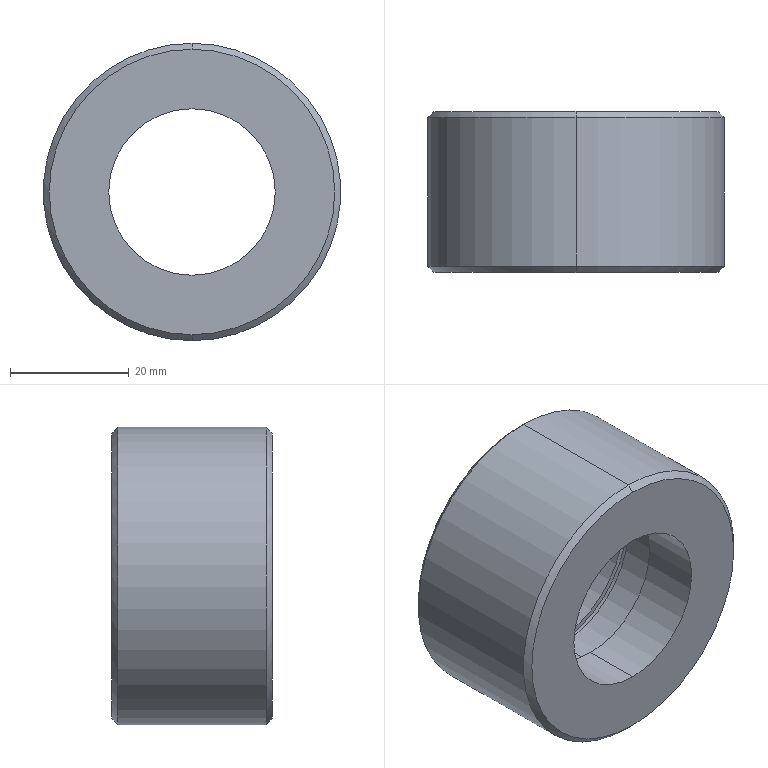Part | SolidWorks | features Chamfer 2, ICE 2, Extrusion 1, RevCut 1 | 1 solid | 21 faces | box 50 x 27 x 50 mm | volume 32903 mm3 | cylinder 10 | cone 6 | plane 5 | commonest cylinder face diameters 32 x4 28 x2 33.7 x2 50 x2
STEP:
#1=CARTESIAN_POINT('',(0.,17.,-16.85));
#2=VERTEX_POINT('',#1);
#3=CARTESIAN_POINT('',(0.,17.,16.85));
#4=VERTEX_POINT('',#3);
#5=CARTESIAN_POINT('',(0.,17.,0.));
#6=DIRECTION('',(0.,1.,0.));
#7=DIRECTION('',(0.,0.,1.));
#8=AXIS2_PLACEMENT_3D('',#5,#6,#7);
#9=CIRCLE('',#8,16.85);
#10=EDGE_CURVE('',#2,#4,#9,.T.);
#11=ORIENTED_EDGE('',*,*,#10,.F.);
#12=CARTESIAN_POINT('',(0.,18.3,-16.85));
#13=VERTEX_POINT('',#12);
#14=CARTESIAN_POINT('',(0.,26.,-16.85));
#15=DIRECTION('',(0.,1.,0.));
#16=VECTOR('',#15,1000.);
#17=LINE('',#14,#16);
#18=EDGE_CURVE('',#2,#13,#17,.T.);
#19=ORIENTED_EDGE('',*,*,#18,.T.);
#20=CARTESIAN_POINT('',(0.,18.3,16.85));
#21=VERTEX_POINT('',#20);
#22=CARTESIAN_POINT('',(0.,18.3,0.));
#23=DIRECTION('',(0.,1.,0.));
#24=DIRECTION('',(0.,0.,1.));
#25=AXIS2_PLACEMENT_3D('',#22,#23,#24);
#26=CIRCLE('',#25,16.85);
#27=EDGE_CURVE('',#13,#21,#26,.T.);
#28=ORIENTED_EDGE('',*,*,#27,.T.);
#29=CARTESIAN_POINT('',(0.,26.,16.85));
#30=DIRECTION('',(0.,1.,0.));
#31=VECTOR('',#30,1000.);
#32=LINE('',#29,#31);
#33=EDGE_CURVE('',#4,#21,#32,.T.);
#34=ORIENTED_EDGE('',*,*,#33,.F.);
#35=EDGE_LOOP('',(#11,#19,#28,#34));
#36=FACE_OUTER_BOUND('',#35,.T.);
#37=CARTESIAN_POINT('',(0.,26.,0.));
#38=DIRECTION('',(0.,1.,0.));
#39=DIRECTION('',(0.,0.,1.));
#40=AXIS2_PLACEMENT_3D('',#37,#38,#39);
#41=CYLINDRICAL_SURFACE('',#40,16.85);
#42=ADVANCED_FACE('',(#36),#41,.F.);
#43=CARTESIAN_POINT('',(0.,26.5,-16.));
#44=VERTEX_POINT('',#43);
#45=CARTESIAN_POINT('',(0.,26.5,16.));
#46=VERTEX_POINT('',#45);
#47=CARTESIAN_POINT('',(0.,26.5,0.));
#48=DIRECTION('',(0.,1.,0.));
#49=DIRECTION('',(0.,0.,1.));
#50=AXIS2_PLACEMENT_3D('',#47,#48,#49);
#51=CIRCLE('',#50,16.);
#52=EDGE_CURVE('',#44,#46,#51,.T.);
#53=ORIENTED_EDGE('',*,*,#52,.F.);
#54=CARTESIAN_POINT('',(0.,27.,-16.5));
#55=VERTEX_POINT('',#54);
#56=CARTESIAN_POINT('',(0.,26.5,-16.));
#57=DIRECTION('',(0.,0.7071,-0.7071));
#58=VECTOR('',#57,1000.);
#59=LINE('',#56,#58);
#60=EDGE_CURVE('',#44,#55,#59,.T.);
#61=ORIENTED_EDGE('',*,*,#60,.T.);
#62=CARTESIAN_POINT('',(0.,27.,16.5));
#63=VERTEX_POINT('',#62);
#64=CARTESIAN_POINT('',(0.,27.,0.));
#65=DIRECTION('',(0.,-1.,0.));
#66=DIRECTION('',(0.,0.,1.));
#67=AXIS2_PLACEMENT_3D('',#64,#65,#66);
#68=CIRCLE('',#67,16.5);
#69=EDGE_CURVE('',#63,#55,#68,.T.);
#70=ORIENTED_EDGE('',*,*,#69,.F.);
#71=CARTESIAN_POINT('',(0.,26.5,16.));
#72=DIRECTION('',(0.,0.7071,0.7071));
#73=VECTOR('',#72,1000.);
#74=LINE('',#71,#73);
#75=EDGE_CURVE('',#46,#63,#74,.T.);
#76=ORIENTED_EDGE('',*,*,#75,.F.);
#77=EDGE_LOOP('',(#53,#61,#70,#76));
#78=FACE_OUTER_BOUND('',#77,.T.);
#79=CARTESIAN_POINT('',(0.,26.5,0.));
#80=DIRECTION('',(0.,1.,0.));
#81=DIRECTION('',(0.,0.,1.));
#82=AXIS2_PLACEMENT_3D('',#79,#80,#81);
#83=CONICAL_SURFACE('',#82,16.,0.7854);
#84=ADVANCED_FACE('',(#78),#83,.F.);
#85=CARTESIAN_POINT('',(0.,27.,24.));
#86=VERTEX_POINT('',#85);
#87=CARTESIAN_POINT('',(0.,27.,-24.));
#88=VERTEX_POINT('',#87);
#89=CARTESIAN_POINT('',(0.,27.,0.));
#90=DIRECTION('',(0.,1.,0.));
#91=DIRECTION('',(0.,0.,1.));
#92=AXIS2_PLACEMENT_3D('',#89,#90,#91);
#93=CIRCLE('',#92,24.);
#94=EDGE_CURVE('',#86,#88,#93,.T.);
#95=ORIENTED_EDGE('',*,*,#94,.F.);
#96=CARTESIAN_POINT('',(0.,26.,25.));
#97=VERTEX_POINT('',#96);
#98=CARTESIAN_POINT('',(0.,27.,24.));
#99=DIRECTION('',(0.,-0.7071,0.7071));
#100=VECTOR('',#99,1000.);
#101=LINE('',#98,#100);
#102=EDGE_CURVE('',#86,#97,#101,.T.);
#103=ORIENTED_EDGE('',*,*,#102,.T.);
#104=CARTESIAN_POINT('',(0.,26.,-25.));
#105=VERTEX_POINT('',#104);
#106=CARTESIAN_POINT('',(0.,26.,0.));
#107=DIRECTION('',(0.,-1.,0.));
#108=DIRECTION('',(0.,0.,1.));
#109=AXIS2_PLACEMENT_3D('',#106,#107,#108);
#110=CIRCLE('',#109,25.);
#111=EDGE_CURVE('',#105,#97,#110,.T.);
#112=ORIENTED_EDGE('',*,*,#111,.F.);
#113=CARTESIAN_POINT('',(0.,27.,-24.));
#114=DIRECTION('',(0.,-0.7071,-0.7071));
#115=VECTOR('',#114,1000.);
#116=LINE('',#113,#115);
#117=EDGE_CURVE('',#88,#105,#116,.T.);
#118=ORIENTED_EDGE('',*,*,#117,.F.);
#119=EDGE_LOOP('',(#95,#103,#112,#118));
#120=FACE_OUTER_BOUND('',#119,.T.);
#121=CARTESIAN_POINT('',(0.,27.,0.));
#122=DIRECTION('',(0.,-1.,0.));
#123=DIRECTION('',(0.,0.,-1.));
#124=AXIS2_PLACEMENT_3D('',#121,#122,#123);
#125=CONICAL_SURFACE('',#124,24.,0.7854);
#126=ADVANCED_FACE('',(#120),#125,.T.);
#127=CARTESIAN_POINT('',(0.,0.,-24.));
#128=VERTEX_POINT('',#127);
#129=CARTESIAN_POINT('',(0.,0.,24.));
#130=VERTEX_POINT('',#129);
#131=CARTESIAN_POINT('',(0.,0.,0.));
#132=DIRECTION('',(0.,-1.,0.));
#133=DIRECTION('',(0.,0.,1.));
#134=AXIS2_PLACEMENT_3D('',#131,#132,#133);
#135=CIRCLE('',#134,24.);
#136=EDGE_CURVE('',#128,#130,#135,.T.);
#137=ORIENTED_EDGE('',*,*,#136,.F.);
#138=CARTESIAN_POINT('',(0.,1.,-25.));
#139=VERTEX_POINT('',#138);
#140=CARTESIAN_POINT('',(0.,1.,-25.));
#141=DIRECTION('',(0.,0.7071,-0.7071));
#142=VECTOR('',#141,1000.);
#143=LINE('',#140,#142);
#144=EDGE_CURVE('',#128,#139,#143,.T.);
#145=ORIENTED_EDGE('',*,*,#144,.T.);
#146=CARTESIAN_POINT('',(0.,1.,25.));
#147=VERTEX_POINT('',#146);
#148=CARTESIAN_POINT('',(0.,1.,0.));
#149=DIRECTION('',(0.,1.,0.));
#150=DIRECTION('',(0.,0.,1.));
#151=AXIS2_PLACEMENT_3D('',#148,#149,#150);
#152=CIRCLE('',#151,25.);
#153=EDGE_CURVE('',#147,#139,#152,.T.);
#154=ORIENTED_EDGE('',*,*,#153,.F.);
#155=CARTESIAN_POINT('',(0.,1.,25.));
#156=DIRECTION('',(0.,0.7071,0.7071));
#157=VECTOR('',#156,1000.);
#158=LINE('',#155,#157);
#159=EDGE_CURVE('',#130,#147,#158,.T.);
#160=ORIENTED_EDGE('',*,*,#159,.F.);
#161=EDGE_LOOP('',(#137,#145,#154,#160));
#162=FACE_OUTER_BOUND('',#161,.T.);
#163=CARTESIAN_POINT('',(0.,1.,0.));
#164=DIRECTION('',(0.,1.,0.));
#165=DIRECTION('',(0.,0.,1.));
#166=AXIS2_PLACEMENT_3D('',#163,#164,#165);
#167=CONICAL_SURFACE('',#166,25.,0.7854);
#168=ADVANCED_FACE('',(#162),#167,.T.);
#169=CARTESIAN_POINT('',(0.,0.,-14.));
#170=VERTEX_POINT('',#169);
#171=CARTESIAN_POINT('',(0.,0.,14.));
#172=VERTEX_POINT('',#171);
#173=CARTESIAN_POINT('',(0.,0.,0.));
#174=DIRECTION('',(0.,1.,0.));
#175=DIRECTION('',(0.,0.,1.));
#176=AXIS2_PLACEMENT_3D('',#173,#174,#175);
#177=CIRCLE('',#176,14.);
#178=EDGE_CURVE('',#170,#172,#177,.T.);
#179=ORIENTED_EDGE('',*,*,#178,.F.);
#180=CARTESIAN_POINT('',(0.,10.,-14.));
#181=VERTEX_POINT('',#180);
#182=CARTESIAN_POINT('',(0.,0.,-14.));
#183=DIRECTION('',(0.,1.,0.));
#184=VECTOR('',#183,1000.);
#185=LINE('',#182,#184);
#186=EDGE_CURVE('',#170,#181,#185,.T.);
#187=ORIENTED_EDGE('',*,*,#186,.T.);
#188=CARTESIAN_POINT('',(0.,10.,14.));
#189=VERTEX_POINT('',#188);
#190=CARTESIAN_POINT('',(0.,10.,0.));
#191=DIRECTION('',(0.,1.,0.));
#192=DIRECTION('',(0.,0.,1.));
#193=AXIS2_PLACEMENT_3D('',#190,#191,#192);
#194=CIRCLE('',#193,14.);
#195=EDGE_CURVE('',#181,#189,#194,.T.);
#196=ORIENTED_EDGE('',*,*,#195,.T.);
#197=CARTESIAN_POINT('',(0.,0.,14.));
#198=DIRECTION('',(0.,1.,0.));
#199=VECTOR('',#198,1000.);
#200=LINE('',#197,#199);
#201=EDGE_CURVE('',#172,#189,#200,.T.);
#202=ORIENTED_EDGE('',*,*,#201,.F.);
#203=EDGE_LOOP('',(#179,#187,#196,#202));
#204=FACE_OUTER_BOUND('',#203,.T.);
#205=CARTESIAN_POINT('',(0.,0.,0.));
#206=DIRECTION('',(0.,1.,0.));
#207=DIRECTION('',(0.,0.,1.));
#208=AXIS2_PLACEMENT_3D('',#205,#206,#207);
#209=CYLINDRICAL_SURFACE('',#208,14.);
#210=ADVANCED_FACE('',(#204),#209,.F.);
#211=CARTESIAN_POINT('',(0.,10.,-16.));
#212=VERTEX_POINT('',#211);
#213=CARTESIAN_POINT('',(0.,10.,16.));
#214=VERTEX_POINT('',#213);
#215=CARTESIAN_POINT('',(0.,10.,0.));
#216=DIRECTION('',(0.,1.,0.));
#217=DIRECTION('',(0.,0.,1.));
#218=AXIS2_PLACEMENT_3D('',#215,#216,#217);
#219=CIRCLE('',#218,16.);
#220=EDGE_CURVE('',#212,#214,#219,.T.);
#221=ORIENTED_EDGE('',*,*,#220,.F.);
#222=CARTESIAN_POINT('',(0.,17.,-16.));
#223=VERTEX_POINT('',#222);
#224=CARTESIAN_POINT('',(0.,10.,-16.));
#225=DIRECTION('',(0.,1.,0.));
#226=VECTOR('',#225,1000.);
#227=LINE('',#224,#226);
#228=EDGE_CURVE('',#212,#223,#227,.T.);
#229=ORIENTED_EDGE('',*,*,#228,.T.);
#230=CARTESIAN_POINT('',(0.,17.,16.));
#231=VERTEX_POINT('',#230);
#232=CARTESIAN_POINT('',(0.,17.,0.));
#233=DIRECTION('',(0.,1.,0.));
#234=DIRECTION('',(0.,0.,-1.));
#235=AXIS2_PLACEMENT_3D('',#232,#233,#234);
#236=CIRCLE('',#235,16.);
#237=EDGE_CURVE('',#223,#231,#236,.T.);
#238=ORIENTED_EDGE('',*,*,#237,.T.);
#239=CARTESIAN_POINT('',(0.,10.,16.));
#240=DIRECTION('',(0.,1.,0.));
#241=VECTOR('',#240,1000.);
#242=LINE('',#239,#241);
#243=EDGE_CURVE('',#214,#231,#242,.T.);
#244=ORIENTED_EDGE('',*,*,#243,.F.);
#245=EDGE_LOOP('',(#221,#229,#238,#244));
#246=FACE_OUTER_BOUND('',#245,.T.);
#247=CARTESIAN_POINT('',(0.,10.,0.));
#248=DIRECTION('',(0.,1.,0.));
#249=DIRECTION('',(0.,0.,1.));
#250=AXIS2_PLACEMENT_3D('',#247,#248,#249);
#251=CYLINDRICAL_SURFACE('',#250,16.);
#252=ADVANCED_FACE('',(#246),#251,.F.);
#253=ORIENTED_EDGE('',*,*,#111,.T.);
#254=CARTESIAN_POINT('',(0.,27.,25.));
#255=DIRECTION('',(0.,-1.,0.));
#256=VECTOR('',#255,1000.);
#257=LINE('',#254,#256);
#258=EDGE_CURVE('',#97,#147,#257,.T.);
#259=ORIENTED_EDGE('',*,*,#258,.T.);
#260=ORIENTED_EDGE('',*,*,#153,.T.);
#261=CARTESIAN_POINT('',(0.,27.,-25.));
#262=DIRECTION('',(0.,-1.,0.));
#263=VECTOR('',#262,1000.);
#264=LINE('',#261,#263);
#265=EDGE_CURVE('',#105,#139,#264,.T.);
#266=ORIENTED_EDGE('',*,*,#265,.F.);
#267=EDGE_LOOP('',(#253,#259,#260,#266));
#268=FACE_OUTER_BOUND('',#267,.T.);
#269=CARTESIAN_POINT('',(0.,27.,0.));
#270=DIRECTION('',(0.,-1.,0.));
#271=DIRECTION('',(0.,0.,-1.));
#272=AXIS2_PLACEMENT_3D('',#269,#270,#271);
#273=CYLINDRICAL_SURFACE('',#272,25.);
#274=ADVANCED_FACE('',(#268),#273,.T.);
#275=CARTESIAN_POINT('',(0.,18.3,16.));
#276=VERTEX_POINT('',#275);
#277=CARTESIAN_POINT('',(0.,18.3,-16.));
#278=VERTEX_POINT('',#277);
#279=CARTESIAN_POINT('',(0.,18.3,0.));
#280=DIRECTION('',(0.,-1.,0.));
#281=DIRECTION('',(0.,0.,1.));
#282=AXIS2_PLACEMENT_3D('',#279,#280,#281);
#283=CIRCLE('',#282,16.);
#284=EDGE_CURVE('',#276,#278,#283,.T.);
#285=ORIENTED_EDGE('',*,*,#284,.T.);
#286=CARTESIAN_POINT('',(0.,10.,-16.));
#287=DIRECTION('',(0.,1.,0.));
#288=VECTOR('',#287,1000.);
#289=LINE('',#286,#288);
#290=EDGE_CURVE('',#278,#44,#289,.T.);
#291=ORIENTED_EDGE('',*,*,#290,.T.);
#292=ORIENTED_EDGE('',*,*,#52,.T.);
#293=CARTESIAN_POINT('',(0.,10.,16.));
#294=DIRECTION('',(0.,1.,0.));
#295=VECTOR('',#294,1000.);
#296=LINE('',#293,#295);
#297=EDGE_CURVE('',#276,#46,#296,.T.);
#298=ORIENTED_EDGE('',*,*,#297,.F.);
#299=EDGE_LOOP('',(#285,#291,#292,#298));
#300=FACE_OUTER_BOUND('',#299,.T.);
#301=CARTESIAN_POINT('',(0.,10.,0.));
#302=DIRECTION('',(0.,1.,0.));
#303=DIRECTION('',(0.,0.,1.));
#304=AXIS2_PLACEMENT_3D('',#301,#302,#303);
#305=CYLINDRICAL_SURFACE('',#304,16.);
#306=ADVANCED_FACE('',(#300),#305,.F.);
#307=ORIENTED_EDGE('',*,*,#290,.F.);
#308=CARTESIAN_POINT('',(0.,18.3,0.));
#309=DIRECTION('',(0.,-1.,0.));
#310=DIRECTION('',(0.,0.,1.));
#311=AXIS2_PLACEMENT_3D('',#308,#309,#310);
#312=CIRCLE('',#311,16.);
#313=EDGE_CURVE('',#278,#276,#312,.T.);
#314=ORIENTED_EDGE('',*,*,#313,.T.);
#315=ORIENTED_EDGE('',*,*,#297,.T.);
#316=CARTESIAN_POINT('',(0.,26.5,0.));
#317=DIRECTION('',(0.,1.,0.));
#318=DIRECTION('',(0.,0.,1.));
#319=AXIS2_PLACEMENT_3D('',#316,#317,#318);
#320=CIRCLE('',#319,16.);
#321=EDGE_CURVE('',#46,#44,#320,.T.);
#322=ORIENTED_EDGE('',*,*,#321,.T.);
#323=EDGE_LOOP('',(#307,#314,#315,#322));
#324=FACE_OUTER_BOUND('',#323,.T.);
#325=CARTESIAN_POINT('',(0.,10.,0.));
#326=DIRECTION('',(0.,1.,0.));
#327=DIRECTION('',(0.,0.,1.));
#328=AXIS2_PLACEMENT_3D('',#325,#326,#327);
#329=CYLINDRICAL_SURFACE('',#328,16.);
#330=ADVANCED_FACE('',(#324),#329,.F.);
#331=ORIENTED_EDGE('',*,*,#258,.F.);
#332=CARTESIAN_POINT('',(0.,26.,0.));
#333=DIRECTION('',(0.,-1.,0.));
#334=DIRECTION('',(0.,0.,1.));
#335=AXIS2_PLACEMENT_3D('',#332,#333,#334);
#336=CIRCLE('',#335,25.);
#337=EDGE_CURVE('',#97,#105,#336,.T.);
#338=ORIENTED_EDGE('',*,*,#337,.T.);
#339=ORIENTED_EDGE('',*,*,#265,.T.);
#340=CARTESIAN_POINT('',(0.,1.,0.));
#341=DIRECTION('',(0.,1.,0.));
#342=DIRECTION('',(0.,0.,1.));
#343=AXIS2_PLACEMENT_3D('',#340,#341,#342);
#344=CIRCLE('',#343,25.);
#345=EDGE_CURVE('',#139,#147,#344,.T.);
#346=ORIENTED_EDGE('',*,*,#345,.T.);
#347=EDGE_LOOP('',(#331,#338,#339,#346));
#348=FACE_OUTER_BOUND('',#347,.T.);
#349=CARTESIAN_POINT('',(0.,27.,0.));
#350=DIRECTION('',(0.,-1.,0.));
#351=DIRECTION('',(0.,0.,-1.));
#352=AXIS2_PLACEMENT_3D('',#349,#350,#351);
#353=CYLINDRICAL_SURFACE('',#352,25.);
#354=ADVANCED_FACE('',(#348),#353,.T.);
#355=ORIENTED_EDGE('',*,*,#69,.T.);
#356=CARTESIAN_POINT('',(0.,27.,0.));
#357=DIRECTION('',(0.,-1.,0.));
#358=DIRECTION('',(0.,0.,1.));
#359=AXIS2_PLACEMENT_3D('',#356,#357,#358);
#360=CIRCLE('',#359,16.5);
#361=EDGE_CURVE('',#55,#63,#360,.T.);
#362=ORIENTED_EDGE('',*,*,#361,.T.);
#363=EDGE_LOOP('',(#355,#362));
#364=FACE_BOUND('',#363,.T.);
#365=CARTESIAN_POINT('',(0.,27.,0.));
#366=DIRECTION('',(0.,1.,0.));
#367=DIRECTION('',(0.,0.,1.));
#368=AXIS2_PLACEMENT_3D('',#365,#366,#367);
#369=CIRCLE('',#368,24.);
#370=EDGE_CURVE('',#88,#86,#369,.T.);
#371=ORIENTED_EDGE('',*,*,#370,.T.);
#372=ORIENTED_EDGE('',*,*,#94,.T.);
#373=EDGE_LOOP('',(#371,#372));
#374=FACE_OUTER_BOUND('',#373,.T.);
#375=CARTESIAN_POINT('',(0.,27.,0.));
#376=DIRECTION('',(0.,1.,0.));
#377=DIRECTION('',(0.,0.,1.));
#378=AXIS2_PLACEMENT_3D('',#375,#376,#377);
#379=PLANE('',#378);
#380=ADVANCED_FACE('',(#364,#374),#379,.T.);
#381=CARTESIAN_POINT('',(0.,0.,0.));
#382=DIRECTION('',(0.,-1.,0.));
#383=DIRECTION('',(0.,0.,1.));
#384=AXIS2_PLACEMENT_3D('',#381,#382,#383);
#385=CIRCLE('',#384,24.);
#386=EDGE_CURVE('',#130,#128,#385,.T.);
#387=ORIENTED_EDGE('',*,*,#386,.T.);
#388=ORIENTED_EDGE('',*,*,#136,.T.);
#389=EDGE_LOOP('',(#387,#388));
#390=FACE_OUTER_BOUND('',#389,.T.);
#391=CARTESIAN_POINT('',(0.,0.,0.));
#392=DIRECTION('',(0.,1.,0.));
#393=DIRECTION('',(0.,0.,1.));
#394=AXIS2_PLACEMENT_3D('',#391,#392,#393);
#395=CIRCLE('',#394,14.);
#396=EDGE_CURVE('',#172,#170,#395,.T.);
#397=ORIENTED_EDGE('',*,*,#396,.T.);
#398=ORIENTED_EDGE('',*,*,#178,.T.);
#399=EDGE_LOOP('',(#397,#398));
#400=FACE_BOUND('',#399,.T.);
#401=CARTESIAN_POINT('',(0.,0.,0.));
#402=DIRECTION('',(0.,1.,0.));
#403=DIRECTION('',(0.,0.,1.));
#404=AXIS2_PLACEMENT_3D('',#401,#402,#403);
#405=PLANE('',#404);
#406=ADVANCED_FACE('',(#390,#400),#405,.F.);
#407=ORIENTED_EDGE('',*,*,#228,.F.);
#408=CARTESIAN_POINT('',(0.,10.,0.));
#409=DIRECTION('',(0.,1.,0.));
#410=DIRECTION('',(0.,0.,1.));
#411=AXIS2_PLACEMENT_3D('',#408,#409,#410);
#412=CIRCLE('',#411,16.);
#413=EDGE_CURVE('',#214,#212,#412,.T.);
#414=ORIENTED_EDGE('',*,*,#413,.F.);
#415=ORIENTED_EDGE('',*,*,#243,.T.);
#416=CARTESIAN_POINT('',(0.,17.,0.));
#417=DIRECTION('',(0.,1.,0.));
#418=DIRECTION('',(0.,0.,-1.));
#419=AXIS2_PLACEMENT_3D('',#416,#417,#418);
#420=CIRCLE('',#419,16.);
#421=EDGE_CURVE('',#231,#223,#420,.T.);
#422=ORIENTED_EDGE('',*,*,#421,.T.);
#423=EDGE_LOOP('',(#407,#414,#415,#422));
#424=FACE_OUTER_BOUND('',#423,.T.);
#425=CARTESIAN_POINT('',(0.,10.,0.));
#426=DIRECTION('',(0.,1.,0.));
#427=DIRECTION('',(0.,0.,1.));
#428=AXIS2_PLACEMENT_3D('',#425,#426,#427);
#429=CYLINDRICAL_SURFACE('',#428,16.);
#430=ADVANCED_FACE('',(#424),#429,.F.);
#431=CARTESIAN_POINT('',(0.,10.,0.));
#432=DIRECTION('',(0.,1.,0.));
#433=DIRECTION('',(0.,0.,1.));
#434=AXIS2_PLACEMENT_3D('',#431,#432,#433);
#435=CIRCLE('',#434,14.);
#436=EDGE_CURVE('',#189,#181,#435,.T.);
#437=ORIENTED_EDGE('',*,*,#436,.F.);
#438=ORIENTED_EDGE('',*,*,#195,.F.);
#439=EDGE_LOOP('',(#437,#438));
#440=FACE_BOUND('',#439,.T.);
#441=ORIENTED_EDGE('',*,*,#413,.T.);
#442=ORIENTED_EDGE('',*,*,#220,.T.);
#443=EDGE_LOOP('',(#441,#442));
#444=FACE_OUTER_BOUND('',#443,.T.);
#445=CARTESIAN_POINT('',(0.,10.,0.));
#446=DIRECTION('',(0.,1.,0.));
#447=DIRECTION('',(0.,0.,1.));
#448=AXIS2_PLACEMENT_3D('',#445,#446,#447);
#449=PLANE('',#448);
#450=ADVANCED_FACE('',(#440,#444),#449,.T.);
#451=ORIENTED_EDGE('',*,*,#186,.F.);
#452=ORIENTED_EDGE('',*,*,#396,.F.);
#453=ORIENTED_EDGE('',*,*,#201,.T.);
#454=ORIENTED_EDGE('',*,*,#436,.T.);
#455=EDGE_LOOP('',(#451,#452,#453,#454));
#456=FACE_OUTER_BOUND('',#455,.T.);
#457=CARTESIAN_POINT('',(0.,0.,0.));
#458=DIRECTION('',(0.,1.,0.));
#459=DIRECTION('',(0.,0.,1.));
#460=AXIS2_PLACEMENT_3D('',#457,#458,#459);
#461=CYLINDRICAL_SURFACE('',#460,14.);
#462=ADVANCED_FACE('',(#456),#461,.F.);
#463=ORIENTED_EDGE('',*,*,#144,.F.);
#464=ORIENTED_EDGE('',*,*,#386,.F.);
#465=ORIENTED_EDGE('',*,*,#159,.T.);
#466=ORIENTED_EDGE('',*,*,#345,.F.);
#467=EDGE_LOOP('',(#463,#464,#465,#466));
#468=FACE_OUTER_BOUND('',#467,.T.);
#469=CARTESIAN_POINT('',(0.,1.,0.));
#470=DIRECTION('',(0.,1.,0.));
#471=DIRECTION('',(0.,0.,1.));
#472=AXIS2_PLACEMENT_3D('',#469,#470,#471);
#473=CONICAL_SURFACE('',#472,25.,0.7854);
#474=ADVANCED_FACE('',(#468),#473,.T.);
#475=ORIENTED_EDGE('',*,*,#102,.F.);
#476=ORIENTED_EDGE('',*,*,#370,.F.);
#477=ORIENTED_EDGE('',*,*,#117,.T.);
#478=ORIENTED_EDGE('',*,*,#337,.F.);
#479=EDGE_LOOP('',(#475,#476,#477,#478));
#480=FACE_OUTER_BOUND('',#479,.T.);
#481=CARTESIAN_POINT('',(0.,27.,0.));
#482=DIRECTION('',(0.,-1.,0.));
#483=DIRECTION('',(0.,0.,-1.));
#484=AXIS2_PLACEMENT_3D('',#481,#482,#483);
#485=CONICAL_SURFACE('',#484,24.,0.7854);
#486=ADVANCED_FACE('',(#480),#485,.T.);
#487=ORIENTED_EDGE('',*,*,#60,.F.);
#488=ORIENTED_EDGE('',*,*,#321,.F.);
#489=ORIENTED_EDGE('',*,*,#75,.T.);
#490=ORIENTED_EDGE('',*,*,#361,.F.);
#491=EDGE_LOOP('',(#487,#488,#489,#490));
#492=FACE_OUTER_BOUND('',#491,.T.);
#493=CARTESIAN_POINT('',(0.,26.5,0.));
#494=DIRECTION('',(0.,1.,0.));
#495=DIRECTION('',(0.,0.,1.));
#496=AXIS2_PLACEMENT_3D('',#493,#494,#495);
#497=CONICAL_SURFACE('',#496,16.,0.7854);
#498=ADVANCED_FACE('',(#492),#497,.F.);
#499=CARTESIAN_POINT('',(0.,18.3,0.));
#500=DIRECTION('',(0.,1.,0.));
#501=DIRECTION('',(0.,0.,1.));
#502=AXIS2_PLACEMENT_3D('',#499,#500,#501);
#503=CIRCLE('',#502,16.85);
#504=EDGE_CURVE('',#21,#13,#503,.T.);
#505=ORIENTED_EDGE('',*,*,#504,.F.);
#506=ORIENTED_EDGE('',*,*,#27,.F.);
#507=EDGE_LOOP('',(#505,#506));
#508=FACE_OUTER_BOUND('',#507,.T.);
#509=ORIENTED_EDGE('',*,*,#284,.F.);
#510=ORIENTED_EDGE('',*,*,#313,.F.);
#511=EDGE_LOOP('',(#509,#510));
#512=FACE_BOUND('',#511,.T.);
#513=CARTESIAN_POINT('',(0.,18.3,16.85));
#514=DIRECTION('',(0.,1.,0.));
#515=DIRECTION('',(0.,0.,1.));
#516=AXIS2_PLACEMENT_3D('',#513,#514,#515);
#517=PLANE('',#516);
#518=ADVANCED_FACE('',(#508,#512),#517,.F.);
#519=CARTESIAN_POINT('',(0.,17.,0.));
#520=DIRECTION('',(0.,1.,0.));
#521=DIRECTION('',(0.,0.,1.));
#522=AXIS2_PLACEMENT_3D('',#519,#520,#521);
#523=CIRCLE('',#522,16.85);
#524=EDGE_CURVE('',#4,#2,#523,.T.);
#525=ORIENTED_EDGE('',*,*,#524,.T.);
#526=ORIENTED_EDGE('',*,*,#10,.T.);
#527=EDGE_LOOP('',(#525,#526));
#528=FACE_OUTER_BOUND('',#527,.T.);
#529=ORIENTED_EDGE('',*,*,#421,.F.);
#530=ORIENTED_EDGE('',*,*,#237,.F.);
#531=EDGE_LOOP('',(#529,#530));
#532=FACE_BOUND('',#531,.T.);
#533=CARTESIAN_POINT('',(0.,17.,16.85));
#534=DIRECTION('',(0.,-1.,0.));
#535=DIRECTION('',(0.,0.,-1.));
#536=AXIS2_PLACEMENT_3D('',#533,#534,#535);
#537=PLANE('',#536);
#538=ADVANCED_FACE('',(#528,#532),#537,.F.);
#539=ORIENTED_EDGE('',*,*,#18,.F.);
#540=ORIENTED_EDGE('',*,*,#524,.F.);
#541=ORIENTED_EDGE('',*,*,#33,.T.);
#542=ORIENTED_EDGE('',*,*,#504,.T.);
#543=EDGE_LOOP('',(#539,#540,#541,#542));
#544=FACE_OUTER_BOUND('',#543,.T.);
#545=CARTESIAN_POINT('',(0.,26.,0.));
#546=DIRECTION('',(0.,1.,0.));
#547=DIRECTION('',(0.,0.,1.));
#548=AXIS2_PLACEMENT_3D('',#545,#546,#547);
#549=CYLINDRICAL_SURFACE('',#548,16.85);
#550=ADVANCED_FACE('',(#544),#549,.F.);
#551=CLOSED_SHELL('',(#42,#84,#126,#168,#210,#252,#274,#306,#330,#354,#380,#406,#430,#450,#462,#474,#486,#498,#518,#538,#550));
#552=MANIFOLD_SOLID_BREP('',#551);
#553=CARTESIAN_POINT('',(0.,0.,0.));
#554=DIRECTION('',(0.,0.,1.));
#555=DIRECTION('',(1.,0.,0.));
#556=AXIS2_PLACEMENT_3D('',#553,#554,#555);
#557=(LENGTH_UNIT()NAMED_UNIT(*)SI_UNIT(.MILLI.,.METRE.));
#558=UNCERTAINTY_MEASURE_WITH_UNIT(LENGTH_MEASURE(0.00001),#557,'','');
#559=(NAMED_UNIT(*)PLANE_ANGLE_UNIT()SI_UNIT($,.RADIAN.));
#560=(NAMED_UNIT(*)SI_UNIT($,.STERADIAN.)SOLID_ANGLE_UNIT());
#561=(GEOMETRIC_REPRESENTATION_CONTEXT(3)GLOBAL_UNCERTAINTY_ASSIGNED_CONTEXT((#558))GLOBAL_UNIT_ASSIGNED_CONTEXT((#557,#559,#560))REPRESENTATION_CONTEXT('',''));
#562=ADVANCED_BREP_SHAPE_REPRESENTATION('',(#552,#556),#561);